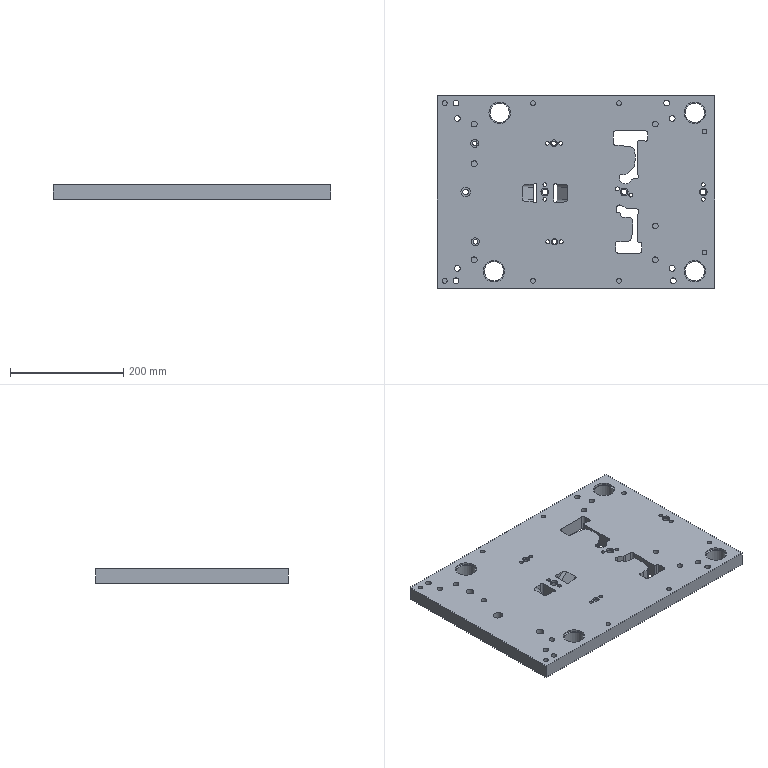Part | NX | features LIN_SOLID_COLOR 2 | 1 solid | 260 faces | box 490 x 340 x 25 mm | volume 3788219 mm3 | plane 132 | cylinder 128 | commonest cylinder face diameters 11 x33 6.8 x10 10.3 x10 6.04 x9 8.5 x8 5.96 x7